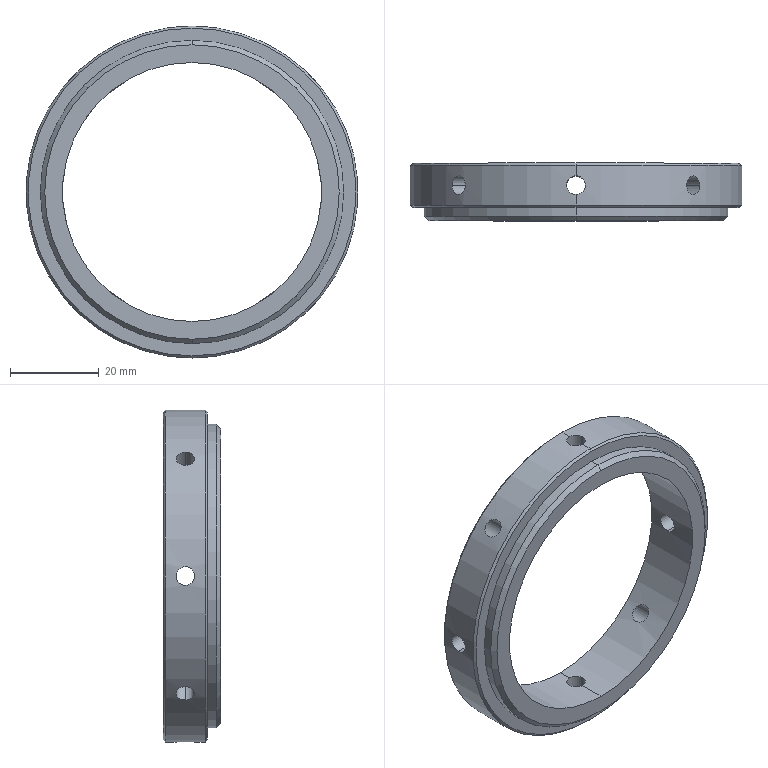Part | SolidWorks | features Chamfer 2, CirPattern 1, Extrusion 1, HoleWzd 1, ICE 1 | 1 solid | 31 faces | box 75 x 13 x 75 mm | volume 19213 mm3 | cylinder 22 | cone 6 | plane 3 | commonest cylinder face diameters 4.2 x16 58.5 x2 68.5 x2 75 x2